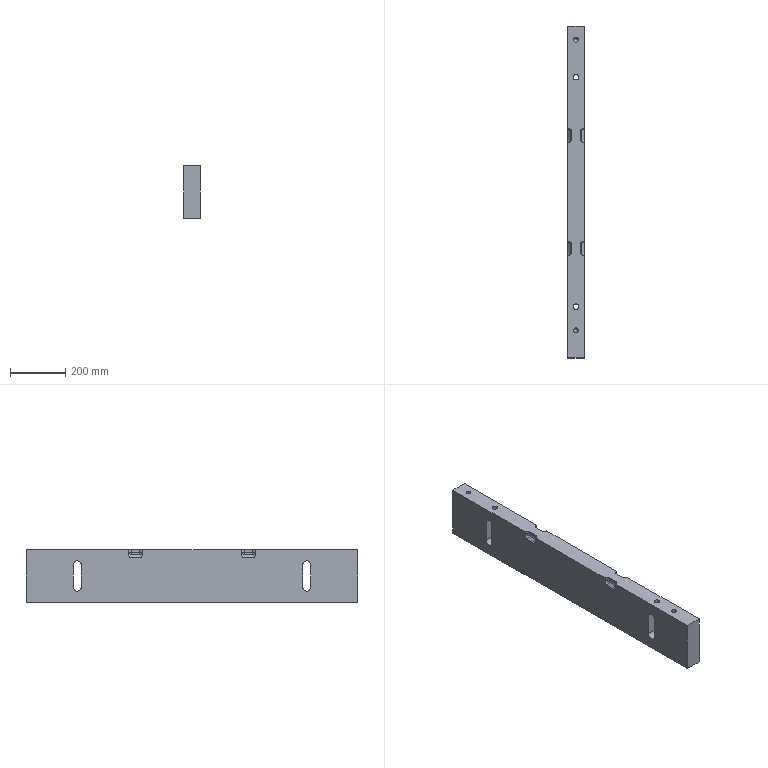Part | STEP file | lll_id4478_x_t | 1 solid | 70 faces | box 60 x 1200 x 190 mm | volume 13159277 mm3 | cylinder 32 | plane 26 | sphere 8 | cone 4 | commonest cylinder face diameters 20 x24 17.506 x4 30 x4